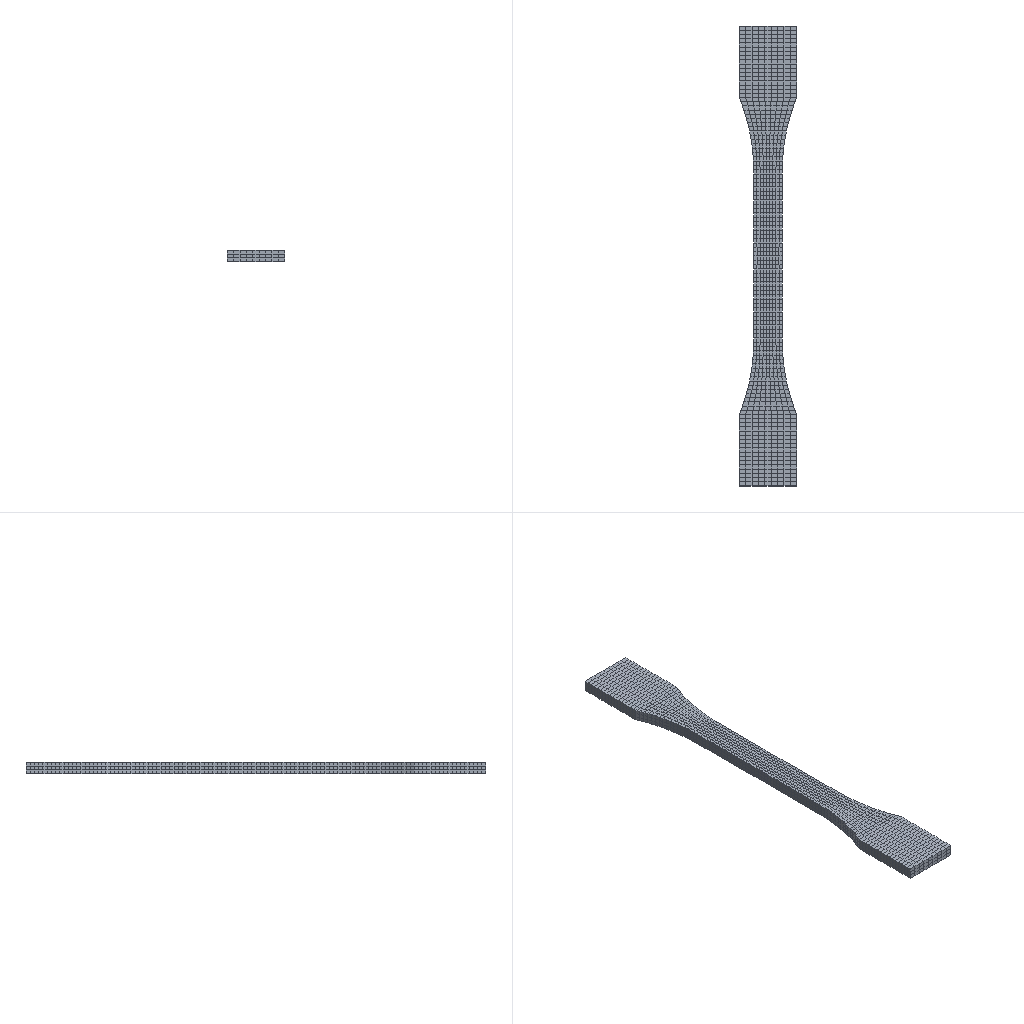Simulation study | abaqus
Set-up summary:
category,name,step,type,value,unit,region
solver,abaqus
solver,version,,,Abaqus/Explicit 3DEXPERIENCE R2017x
units,not stated in the deck,,not stated
analysis,deck,,transient,transient
load_step,Step-1,Step-1,transient,nlgeom=True
contact,interactions,,,general=0 pairs=0 ties=0
load_step,requested,,,1
mesh,nodes,,,4360
mesh,elements,,,2916
element_type,C3D8R,,solid,2916
load,load commands in deck,,count,1
bc,support commands in deck,,count,7
material,MATERIAL-1,,in results
check,setup vs results,,match,"per instance, exact: element labels, types and connectivity; labels of the nodes the elements use; coordinates of those nodes at SINGLE_PRECISION in 1 of 1 instance(s)"
Abaqus input file, long lists of numbers shortened:
*Heading
** Job name: Job-1 Model name: Model-1
** Generated by: Abaqus/CAE 2017
*Preprint, echo=NO, model=NO, history=NO, contact=NO
**
** PARTS
**
*Part, name=work
*Node
      1,           5.,         -30.,           4.
      2,          10.,         -55.,           4.
** (4358 more lines like these left out)
*Element, type=C3D8R
  1,  113,  693, 2745,  661,    1,   33,  597,   68
  2,  693,  694, 2746, 2745,   33,   34,  598,  597
** (2914 more lines like these left out)
*Nset, nset=Set-1, generate
    1,  4360,     1
*Elset, elset=Set-1, generate
    1,  2916,     1
** Section: Section-1
*Solid Section, elset=Set-1, material=Material-1
,
*End Part
**
**
** ASSEMBLY
**
*Assembly, name=Assembly
**
*Instance, name=work-1, part=work
*End Instance
**
*Nset, nset=Set-1, instance=work-1, generate
    1,  4360,     1
*Elset, elset=Set-1, instance=work-1, generate
    1,  2916,     1
*Nset, nset=Set-2, instance=work-1
   21,   22,   23,   24,  305,  306,  339,  340,  357,  358,  359,  360,  361,  362,  363,  364
  365,  366,  367,  368,  369,  370,  371,  372, 1521, 1522, 1523, 1524, 1525, 1526, 1527, 1528
** (1 more lines like these left out)
*Elset, elset=Set-2, instance=work-1, generate
 1151,  1593,    17
*Nset, nset=Set-3, instance=work-1
    2,    3,    5,    6,   21,   22,   23,   24,   49,   50,   85,   86,  121,  122,  123,  124
  125,  126,  127,  128,  129,  130,  131,  132,  133,  134,  135,  136,  289,  290,  291,  292
** (43 more lines like these left out)
*Elset, elset=Set-3, instance=work-1, generate
 1135,  1593,     1
*Nset, nset=Set-4, instance=work-1
   25,   26,   27,   28,   29,   30,   31,   32,  373,  374,  375,  376,  377,  378,  379,  380
  381,  382,  383,  384,  385,  386,  387,  388,  389,  390,  391,  392,  393,  394,  395,  396
** (43 more lines like these left out)
*Elset, elset=Set-4, instance=work-1, generate
 1594,  2052,     1
*End Assembly
**
** MATERIALS
**
*Material, name=Material-1
*Conductivity
 0.25,
*Density
 1.2e-09,
*Depvar, delete=10
     13,
*Specific Heat
 1.17e+09,
*User Material, constants=25
2200.,     0.39,    -62.7,   -30.99,  -1.859,     2.46,    -1.62,     4.54
   0.2724,       0.,     2.35,     0.63,       1.,   0.0014,     398.,     413.
      0.9, 1.17e+09,       0.,   27000.,     170.,      50.,      70.,      50.
      70.,
**
** PREDEFINED FIELDS
**
** Name: Predefined Field-1   Type: Temperature
*Initial Conditions, type=TEMPERATURE
Set-1, 398.
** ----------------------------------------------------------------
**
** STEP: Step-1
**
*Step, name=Step-1, nlgeom=YES
*Dynamic, Explicit
, 0.06
*Bulk Viscosity
0.06, 1.2
**
** BOUNDARY CONDITIONS
**
** Name: BC-1 Type: 对称/反对称/完全固定
*Boundary
Set-3, ENCASTRE
** Name: [REDACTED] : Velocity/Angular velocity
*Boundary, type=VELOCITY
Set-4, 1, 1
Set-4, 2, 2, 833.
Set-4, 3, 3
Set-4, 4, 4
Set-4, 5, 5
Set-4, 6, 6
**
** OUTPUT REQUESTS
**
*Restart, write, number interval=1, time marks=NO
**
** FIELD OUTPUT: F-Output-1
**
*Output, field, number interval=30
*Node Output
A, CF, RF, RM, RT, U, V
*Element Output, directions=YES
E, FV, LE, MFR, MISES, MISESMAX, MISESONLY, PE, PEEQ, PEEQMAX, PEEQT, PEEQVAVG, PEMAG, PEVAVG, PRESSONLY, S
SDV, SFABRIC, SSAVG, STATUS, SVAVG, TEMP, UVARM, VEEQ
*Contact Output
CDISP, CSTRESS
**
** HISTORY OUTPUT: H-Output-1
**
*Output, history, variable=PRESELECT
*End Step
Results summary:
result,step,Step-1,completed,increments=192340 time=0.06/0.06
result,analysis,,,transient
result,last_loadstep,,,1
result,analysis steps,,count,1
result,primary field,,,U
result,reaction total,,FX,-0.05465,model units
result,reaction total,,FY,-0.3888,model units
result,reaction total,,FZ,-0.6768,model units